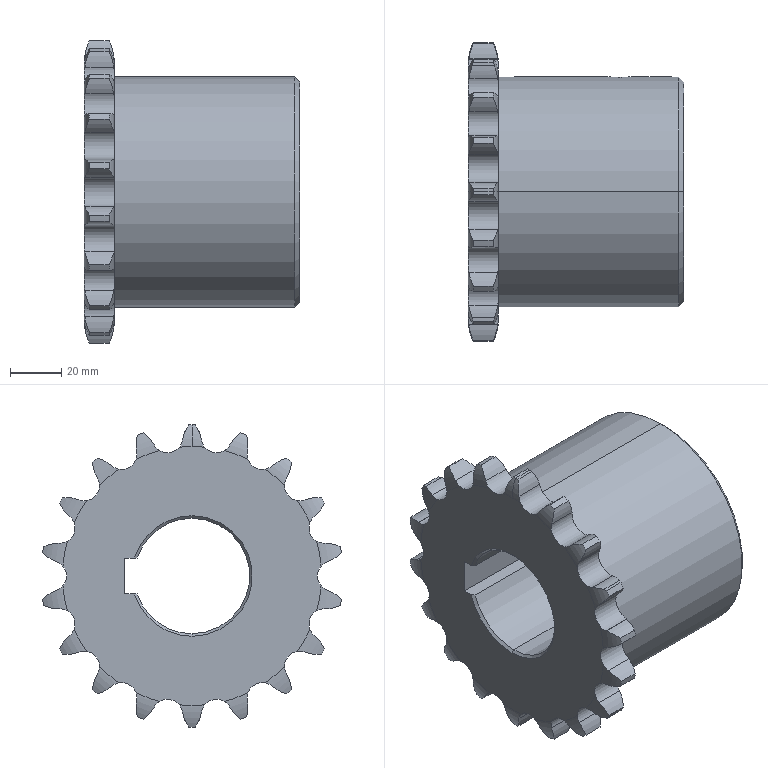Part | SolidWorks | features ICE 2, Chamfer 1, CirPattern 1, HoleWzd 1, RefAxis 1, Revolution 1 | 1 solid | 144 faces | box 84 x 116.518 x 117.9 mm | volume 421510 mm3 | cylinder 92 | torus 38 | cone 8 | plane 6 | commonest cylinder face diameters 28 x40 11.91 x26 117.9 x19 45 x3 10.2 x2 90 x2